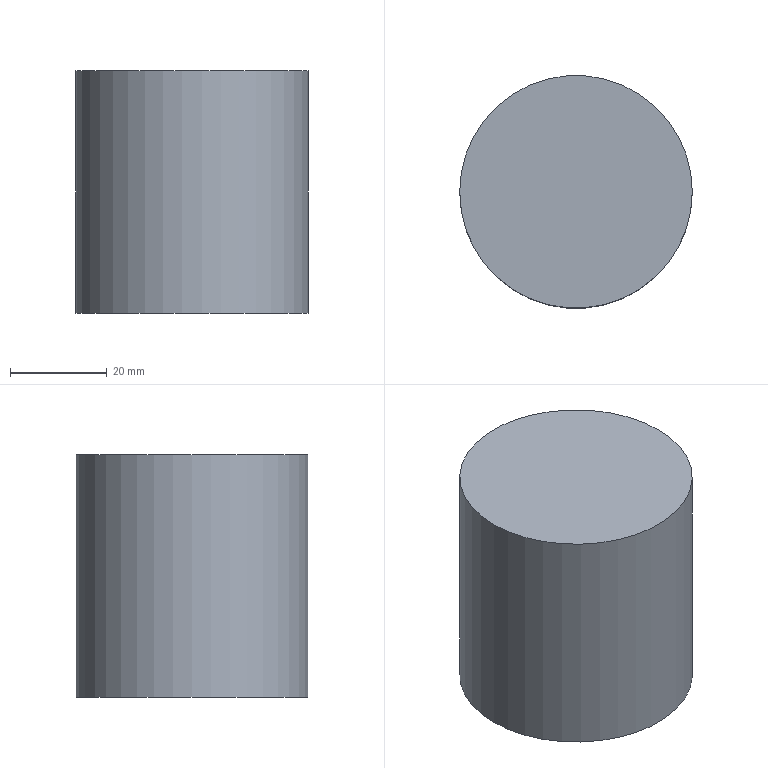Part | STEP file | UPPER ELECTRODE PROJECTION 1 | 1 solid | 3 faces | box 48 x 48 x 50 mm | volume 90478 mm3 | plane 2 | cylinder 1 | commonest cylinder face diameters 48 x1
STEP:
#1=CARTESIAN_POINT('',(0.,0.,0.));
#2=DIRECTION('',(0.,0.,1.));
#3=DIRECTION('',(1.,0.,0.));
#4=AXIS2_PLACEMENT_3D('',#1,#2,#3);
#5=CARTESIAN_POINT('',(24.,0.,50.));
#6=VERTEX_POINT('',#5);
#7=CARTESIAN_POINT('',(0.,0.,50.));
#8=DIRECTION('',(0.,0.,-1.));
#9=DIRECTION('',(-1.,0.,0.));
#10=AXIS2_PLACEMENT_3D('',#7,#8,#9);
#11=CIRCLE('',#10,24.);
#12=CARTESIAN_POINT('',(0.,0.,0.));
#13=DIRECTION('',(0.,0.,1.));
#14=DIRECTION('',(-1.,0.,0.));
#15=AXIS2_PLACEMENT_3D('',#12,#13,#14);
#16=CYLINDRICAL_SURFACE('',#15,24.);
#17=CARTESIAN_POINT('',(12.566,50.));
#18=DIRECTION('',(-1.,0.));
#19=VECTOR('',#18,1.);
#20=LINE('',#17,#19);
#21=(GEOMETRIC_REPRESENTATION_CONTEXT(2)PARAMETRIC_REPRESENTATION_CONTEXT()REPRESENTATION_CONTEXT('',''));
#22=DEFINITIONAL_REPRESENTATION('',(#20),#21);
#23=PCURVE('',#16,#22);
#24=CARTESIAN_POINT('',(0.,0.,50.));
#25=DIRECTION('',(0.,0.,-1.));
#26=DIRECTION('',(-1.,0.,0.));
#27=AXIS2_PLACEMENT_3D('',#24,#25,#26);
#28=PLANE('',#27);
#29=CARTESIAN_POINT('',(0.,0.));
#30=DIRECTION('',(1.,0.));
#31=AXIS2_PLACEMENT_2D('',#29,#30);
#32=CIRCLE('',#31,24.);
#33=(GEOMETRIC_REPRESENTATION_CONTEXT(2)PARAMETRIC_REPRESENTATION_CONTEXT()REPRESENTATION_CONTEXT('',''));
#34=DEFINITIONAL_REPRESENTATION('',(#32),#33);
#35=PCURVE('',#28,#34);
#36=SURFACE_CURVE('',#11,(#23,#35),.PCURVE_S1.);
#37=EDGE_CURVE('',#6,#6,#36,.T.);
#38=ORIENTED_EDGE('',*,*,#37,.T.);
#39=CARTESIAN_POINT('',(24.,0.,0.));
#40=VERTEX_POINT('',#39);
#41=CARTESIAN_POINT('',(24.,0.,0.));
#42=CARTESIAN_POINT('',(24.,0.,50.));
#43=B_SPLINE_CURVE_WITH_KNOTS('',1,(#41,#42),.UNSPECIFIED.,.F.,.F.,(2,2),(0.,50.),.PIECEWISE_BEZIER_KNOTS.);
#44=CARTESIAN_POINT('',(3.142,0.));
#45=DIRECTION('',(0.,1.));
#46=VECTOR('',#45,1.);
#47=LINE('',#44,#46);
#48=(GEOMETRIC_REPRESENTATION_CONTEXT(2)PARAMETRIC_REPRESENTATION_CONTEXT()REPRESENTATION_CONTEXT('',''));
#49=DEFINITIONAL_REPRESENTATION('',(#47),#48);
#50=PCURVE('',#16,#49);
#51=CARTESIAN_POINT('',(9.425,0.));
#52=DIRECTION('',(0.,1.));
#53=VECTOR('',#52,1.);
#54=LINE('',#51,#53);
#55=(GEOMETRIC_REPRESENTATION_CONTEXT(2)PARAMETRIC_REPRESENTATION_CONTEXT()REPRESENTATION_CONTEXT('',''));
#56=DEFINITIONAL_REPRESENTATION('',(#54),#55);
#57=PCURVE('',#16,#56);
#58=SEAM_CURVE('',#43,(#50,#57),.PCURVE_S1.);
#59=EDGE_CURVE('',#40,#6,#58,.T.);
#60=ORIENTED_EDGE('',*,*,#59,.F.);
#61=CARTESIAN_POINT('',(0.,0.,0.));
#62=DIRECTION('',(0.,0.,-1.));
#63=DIRECTION('',(-1.,0.,0.));
#64=AXIS2_PLACEMENT_3D('',#61,#62,#63);
#65=CIRCLE('',#64,24.);
#66=CARTESIAN_POINT('',(12.566,0.));
#67=DIRECTION('',(-1.,0.));
#68=VECTOR('',#67,1.);
#69=LINE('',#66,#68);
#70=(GEOMETRIC_REPRESENTATION_CONTEXT(2)PARAMETRIC_REPRESENTATION_CONTEXT()REPRESENTATION_CONTEXT('',''));
#71=DEFINITIONAL_REPRESENTATION('',(#69),#70);
#72=PCURVE('',#16,#71);
#73=CARTESIAN_POINT('',(0.,0.,0.));
#74=DIRECTION('',(0.,0.,-1.));
#75=DIRECTION('',(-1.,0.,0.));
#76=AXIS2_PLACEMENT_3D('',#73,#74,#75);
#77=PLANE('',#76);
#78=CARTESIAN_POINT('',(0.,0.));
#79=DIRECTION('',(1.,0.));
#80=AXIS2_PLACEMENT_2D('',#78,#79);
#81=CIRCLE('',#80,24.);
#82=(GEOMETRIC_REPRESENTATION_CONTEXT(2)PARAMETRIC_REPRESENTATION_CONTEXT()REPRESENTATION_CONTEXT('',''));
#83=DEFINITIONAL_REPRESENTATION('',(#81),#82);
#84=PCURVE('',#77,#83);
#85=SURFACE_CURVE('',#65,(#72,#84),.PCURVE_S1.);
#86=EDGE_CURVE('',#40,#40,#85,.T.);
#87=ORIENTED_EDGE('',*,*,#86,.F.);
#88=ORIENTED_EDGE('',*,*,#59,.T.);
#89=EDGE_LOOP('',(#38,#60,#87,#88));
#90=FACE_BOUND('',#89,.T.);
#91=ADVANCED_FACE('',(#90),#16,.T.);
#92=ORIENTED_EDGE('',*,*,#37,.F.);
#93=EDGE_LOOP('',(#92));
#94=FACE_BOUND('',#93,.T.);
#95=ADVANCED_FACE('',(#94),#28,.F.);
#96=ORIENTED_EDGE('',*,*,#86,.T.);
#97=EDGE_LOOP('',(#96));
#98=FACE_BOUND('',#97,.T.);
#99=ADVANCED_FACE('',(#98),#77,.T.);
#100=CLOSED_SHELL('',(#91,#95,#99));
#101=MANIFOLD_SOLID_BREP('',#100);
#102=(LENGTH_UNIT()NAMED_UNIT(*)SI_UNIT(.MILLI.,.METRE.));
#103=UNCERTAINTY_MEASURE_WITH_UNIT(LENGTH_MEASURE(0.00001),#102,'','');
#104=(NAMED_UNIT(*)PLANE_ANGLE_UNIT()SI_UNIT($,.RADIAN.));
#105=(NAMED_UNIT(*)SI_UNIT($,.STERADIAN.)SOLID_ANGLE_UNIT());
#106=(GEOMETRIC_REPRESENTATION_CONTEXT(3)GLOBAL_UNCERTAINTY_ASSIGNED_CONTEXT((#103))GLOBAL_UNIT_ASSIGNED_CONTEXT((#102,#104,#105))REPRESENTATION_CONTEXT('',''));
#107=ADVANCED_BREP_SHAPE_REPRESENTATION('',(#4,#101),#106);